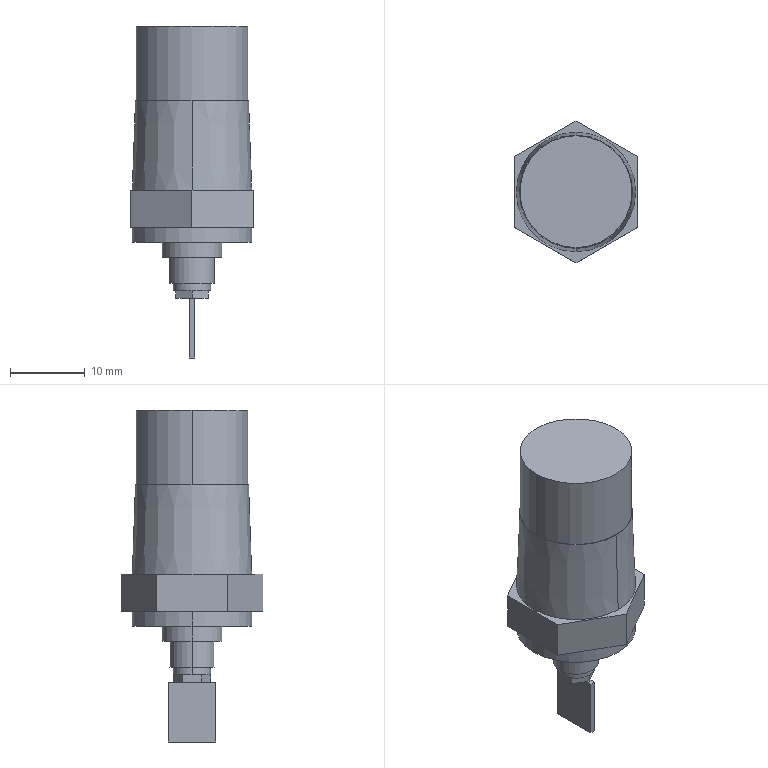Part | SolidWorks | features BaseBody 1 | 1 solid | 46 faces | box 16.454 x 19 x 44.5 mm | volume 5901 mm3 | plane 34 | cylinder 10 | cone 2 | commonest cylinder face diameters 5 x2 6 x2 8 x2 15 x2 16 x2
STEP:
#1=CARTESIAN_POINT('',(0.,7.581,0.));
#2=VERTEX_POINT('',#1);
#3=CARTESIAN_POINT('',(0.,-7.581,0.));
#4=VERTEX_POINT('',#3);
#5=CARTESIAN_POINT('',(0.,0.,0.));
#6=DIRECTION('',(0.,0.,-1.));
#7=DIRECTION('',(0.,1.,0.));
#8=AXIS2_PLACEMENT_3D('',#5,#6,#7);
#9=CIRCLE('',#8,7.581);
#10=EDGE_CURVE('',#2,#4,#9,.T.);
#11=ORIENTED_EDGE('',*,*,#10,.T.);
#12=CARTESIAN_POINT('',(0.,-8.,-12.));
#13=VERTEX_POINT('',#12);
#14=CARTESIAN_POINT('',(0.,-8.,-12.));
#15=DIRECTION('',(0.,-0.0349,-0.9994));
#16=VECTOR('',#15,1000.);
#17=LINE('',#14,#16);
#18=EDGE_CURVE('',#4,#13,#17,.T.);
#19=ORIENTED_EDGE('',*,*,#18,.T.);
#20=CARTESIAN_POINT('',(0.,8.,-12.));
#21=VERTEX_POINT('',#20);
#22=CARTESIAN_POINT('',(0.,0.,-12.));
#23=DIRECTION('',(0.,0.,1.));
#24=DIRECTION('',(0.,1.,0.));
#25=AXIS2_PLACEMENT_3D('',#22,#23,#24);
#26=CIRCLE('',#25,8.);
#27=EDGE_CURVE('',#13,#21,#26,.T.);
#28=ORIENTED_EDGE('',*,*,#27,.T.);
#29=CARTESIAN_POINT('',(0.,8.,-12.));
#30=DIRECTION('',(0.,0.0349,-0.9994));
#31=VECTOR('',#30,1000.);
#32=LINE('',#29,#31);
#33=EDGE_CURVE('',#2,#21,#32,.T.);
#34=ORIENTED_EDGE('',*,*,#33,.F.);
#35=EDGE_LOOP('',(#11,#19,#28,#34));
#36=FACE_OUTER_BOUND('',#35,.T.);
#37=CARTESIAN_POINT('',(0.,0.,-12.));
#38=DIRECTION('',(0.,0.,-1.));
#39=DIRECTION('',(0.,1.,0.));
#40=AXIS2_PLACEMENT_3D('',#37,#38,#39);
#41=CONICAL_SURFACE('',#40,8.,0.03491);
#42=ADVANCED_FACE('',(#36),#41,.T.);
#43=CARTESIAN_POINT('',(-7.5,0.,0.));
#44=VERTEX_POINT('',#43);
#45=CARTESIAN_POINT('',(7.5,0.,0.));
#46=VERTEX_POINT('',#45);
#47=CARTESIAN_POINT('',(0.,0.,0.));
#48=DIRECTION('',(0.,0.,-1.));
#49=DIRECTION('',(1.,0.,0.));
#50=AXIS2_PLACEMENT_3D('',#47,#48,#49);
#51=CIRCLE('',#50,7.5);
#52=EDGE_CURVE('',#44,#46,#51,.T.);
#53=ORIENTED_EDGE('',*,*,#52,.F.);
#54=CARTESIAN_POINT('',(-7.5,0.,10.));
#55=VERTEX_POINT('',#54);
#56=CARTESIAN_POINT('',(-7.5,0.,0.));
#57=DIRECTION('',(0.,0.,1.));
#58=VECTOR('',#57,1000.);
#59=LINE('',#56,#58);
#60=EDGE_CURVE('',#44,#55,#59,.T.);
#61=ORIENTED_EDGE('',*,*,#60,.T.);
#62=CARTESIAN_POINT('',(7.5,0.,10.));
#63=VERTEX_POINT('',#62);
#64=CARTESIAN_POINT('',(0.,0.,10.));
#65=DIRECTION('',(0.,0.,-1.));
#66=DIRECTION('',(1.,0.,0.));
#67=AXIS2_PLACEMENT_3D('',#64,#65,#66);
#68=CIRCLE('',#67,7.5);
#69=EDGE_CURVE('',#55,#63,#68,.T.);
#70=ORIENTED_EDGE('',*,*,#69,.T.);
#71=CARTESIAN_POINT('',(7.5,0.,0.));
#72=DIRECTION('',(0.,0.,1.));
#73=VECTOR('',#72,1000.);
#74=LINE('',#71,#73);
#75=EDGE_CURVE('',#46,#63,#74,.T.);
#76=ORIENTED_EDGE('',*,*,#75,.F.);
#77=EDGE_LOOP('',(#53,#61,#70,#76));
#78=FACE_OUTER_BOUND('',#77,.T.);
#79=CARTESIAN_POINT('',(0.,0.,0.));
#80=DIRECTION('',(0.,0.,1.));
#81=DIRECTION('',(1.,0.,0.));
#82=AXIS2_PLACEMENT_3D('',#79,#80,#81);
#83=CYLINDRICAL_SURFACE('',#82,7.5);
#84=ADVANCED_FACE('',(#78),#83,.T.);
#85=CARTESIAN_POINT('',(-8.,0.,-17.));
#86=VERTEX_POINT('',#85);
#87=CARTESIAN_POINT('',(8.,0.,-17.));
#88=VERTEX_POINT('',#87);
#89=CARTESIAN_POINT('',(0.,0.,-17.));
#90=DIRECTION('',(0.,0.,-1.));
#91=DIRECTION('',(-1.,0.,0.));
#92=AXIS2_PLACEMENT_3D('',#89,#90,#91);
#93=CIRCLE('',#92,8.);
#94=EDGE_CURVE('',#86,#88,#93,.T.);
#95=ORIENTED_EDGE('',*,*,#94,.T.);
#96=CARTESIAN_POINT('',(8.,0.,-19.));
#97=VERTEX_POINT('',#96);
#98=CARTESIAN_POINT('',(8.,0.,-17.));
#99=DIRECTION('',(0.,0.,-1.));
#100=VECTOR('',#99,1000.);
#101=LINE('',#98,#100);
#102=EDGE_CURVE('',#88,#97,#101,.T.);
#103=ORIENTED_EDGE('',*,*,#102,.T.);
#104=CARTESIAN_POINT('',(-8.,0.,-19.));
#105=VERTEX_POINT('',#104);
#106=CARTESIAN_POINT('',(0.,0.,-19.));
#107=DIRECTION('',(0.,0.,1.));
#108=DIRECTION('',(-1.,0.,0.));
#109=AXIS2_PLACEMENT_3D('',#106,#107,#108);
#110=CIRCLE('',#109,8.);
#111=EDGE_CURVE('',#97,#105,#110,.T.);
#112=ORIENTED_EDGE('',*,*,#111,.T.);
#113=CARTESIAN_POINT('',(-8.,0.,-17.));
#114=DIRECTION('',(0.,0.,-1.));
#115=VECTOR('',#114,1000.);
#116=LINE('',#113,#115);
#117=EDGE_CURVE('',#86,#105,#116,.T.);
#118=ORIENTED_EDGE('',*,*,#117,.F.);
#119=EDGE_LOOP('',(#95,#103,#112,#118));
#120=FACE_OUTER_BOUND('',#119,.T.);
#121=CARTESIAN_POINT('',(0.,0.,-17.));
#122=DIRECTION('',(0.,0.,-1.));
#123=DIRECTION('',(-1.,0.,0.));
#124=AXIS2_PLACEMENT_3D('',#121,#122,#123);
#125=CYLINDRICAL_SURFACE('',#124,8.);
#126=ADVANCED_FACE('',(#120),#125,.T.);
#127=CARTESIAN_POINT('',(-4.,0.,-19.));
#128=VERTEX_POINT('',#127);
#129=CARTESIAN_POINT('',(4.,0.,-19.));
#130=VERTEX_POINT('',#129);
#131=CARTESIAN_POINT('',(0.,0.,-19.));
#132=DIRECTION('',(0.,0.,-1.));
#133=DIRECTION('',(-1.,0.,0.));
#134=AXIS2_PLACEMENT_3D('',#131,#132,#133);
#135=CIRCLE('',#134,4.);
#136=EDGE_CURVE('',#128,#130,#135,.T.);
#137=ORIENTED_EDGE('',*,*,#136,.T.);
#138=CARTESIAN_POINT('',(4.,0.,-21.));
#139=VERTEX_POINT('',#138);
#140=CARTESIAN_POINT('',(4.,0.,-19.));
#141=DIRECTION('',(0.,0.,-1.));
#142=VECTOR('',#141,1000.);
#143=LINE('',#140,#142);
#144=EDGE_CURVE('',#130,#139,#143,.T.);
#145=ORIENTED_EDGE('',*,*,#144,.T.);
#146=CARTESIAN_POINT('',(-4.,0.,-21.));
#147=VERTEX_POINT('',#146);
#148=CARTESIAN_POINT('',(0.,0.,-21.));
#149=DIRECTION('',(0.,0.,1.));
#150=DIRECTION('',(-1.,0.,0.));
#151=AXIS2_PLACEMENT_3D('',#148,#149,#150);
#152=CIRCLE('',#151,4.);
#153=EDGE_CURVE('',#139,#147,#152,.T.);
#154=ORIENTED_EDGE('',*,*,#153,.T.);
#155=CARTESIAN_POINT('',(-4.,0.,-19.));
#156=DIRECTION('',(0.,0.,-1.));
#157=VECTOR('',#156,1000.);
#158=LINE('',#155,#157);
#159=EDGE_CURVE('',#128,#147,#158,.T.);
#160=ORIENTED_EDGE('',*,*,#159,.F.);
#161=EDGE_LOOP('',(#137,#145,#154,#160));
#162=FACE_OUTER_BOUND('',#161,.T.);
#163=CARTESIAN_POINT('',(0.,0.,-19.));
#164=DIRECTION('',(0.,0.,-1.));
#165=DIRECTION('',(-1.,0.,0.));
#166=AXIS2_PLACEMENT_3D('',#163,#164,#165);
#167=CYLINDRICAL_SURFACE('',#166,4.);
#168=ADVANCED_FACE('',(#162),#167,.T.);
#169=CARTESIAN_POINT('',(-3.,0.,-21.));
#170=VERTEX_POINT('',#169);
#171=CARTESIAN_POINT('',(3.,0.,-21.));
#172=VERTEX_POINT('',#171);
#173=CARTESIAN_POINT('',(0.,0.,-21.));
#174=DIRECTION('',(0.,0.,-1.));
#175=DIRECTION('',(-1.,0.,0.));
#176=AXIS2_PLACEMENT_3D('',#173,#174,#175);
#177=CIRCLE('',#176,3.);
#178=EDGE_CURVE('',#170,#172,#177,.T.);
#179=ORIENTED_EDGE('',*,*,#178,.T.);
#180=CARTESIAN_POINT('',(3.,0.,-24.5));
#181=VERTEX_POINT('',#180);
#182=CARTESIAN_POINT('',(3.,0.,-21.));
#183=DIRECTION('',(0.,0.,-1.));
#184=VECTOR('',#183,1000.);
#185=LINE('',#182,#184);
#186=EDGE_CURVE('',#172,#181,#185,.T.);
#187=ORIENTED_EDGE('',*,*,#186,.T.);
#188=CARTESIAN_POINT('',(-3.,0.,-24.5));
#189=VERTEX_POINT('',#188);
#190=CARTESIAN_POINT('',(0.,0.,-24.5));
#191=DIRECTION('',(0.,0.,1.));
#192=DIRECTION('',(-1.,0.,0.));
#193=AXIS2_PLACEMENT_3D('',#190,#191,#192);
#194=CIRCLE('',#193,3.);
#195=EDGE_CURVE('',#181,#189,#194,.T.);
#196=ORIENTED_EDGE('',*,*,#195,.T.);
#197=CARTESIAN_POINT('',(-3.,0.,-21.));
#198=DIRECTION('',(0.,0.,-1.));
#199=VECTOR('',#198,1000.);
#200=LINE('',#197,#199);
#201=EDGE_CURVE('',#170,#189,#200,.T.);
#202=ORIENTED_EDGE('',*,*,#201,.F.);
#203=EDGE_LOOP('',(#179,#187,#196,#202));
#204=FACE_OUTER_BOUND('',#203,.T.);
#205=CARTESIAN_POINT('',(0.,0.,-21.));
#206=DIRECTION('',(0.,0.,-1.));
#207=DIRECTION('',(-1.,0.,0.));
#208=AXIS2_PLACEMENT_3D('',#205,#206,#207);
#209=CYLINDRICAL_SURFACE('',#208,3.);
#210=ADVANCED_FACE('',(#204),#209,.T.);
#211=CARTESIAN_POINT('',(-2.5,0.,-24.5));
#212=VERTEX_POINT('',#211);
#213=CARTESIAN_POINT('',(2.5,0.,-24.5));
#214=VERTEX_POINT('',#213);
#215=CARTESIAN_POINT('',(0.,0.,-24.5));
#216=DIRECTION('',(0.,0.,-1.));
#217=DIRECTION('',(-1.,0.,0.));
#218=AXIS2_PLACEMENT_3D('',#215,#216,#217);
#219=CIRCLE('',#218,2.5);
#220=EDGE_CURVE('',#212,#214,#219,.T.);
#221=ORIENTED_EDGE('',*,*,#220,.T.);
#222=CARTESIAN_POINT('',(2.5,0.,-25.5));
#223=VERTEX_POINT('',#222);
#224=CARTESIAN_POINT('',(2.5,0.,-24.5));
#225=DIRECTION('',(0.,0.,-1.));
#226=VECTOR('',#225,1000.);
#227=LINE('',#224,#226);
#228=EDGE_CURVE('',#214,#223,#227,.T.);
#229=ORIENTED_EDGE('',*,*,#228,.T.);
#230=CARTESIAN_POINT('',(2.165,1.25,-25.5));
#231=VERTEX_POINT('',#230);
#232=CARTESIAN_POINT('',(0.,0.,-25.5));
#233=DIRECTION('',(0.,0.,1.));
#234=DIRECTION('',(-1.,0.,0.));
#235=AXIS2_PLACEMENT_3D('',#232,#233,#234);
#236=CIRCLE('',#235,2.5);
#237=EDGE_CURVE('',#223,#231,#236,.T.);
#238=ORIENTED_EDGE('',*,*,#237,.T.);
#239=CARTESIAN_POINT('',(0.,2.5,-25.5));
#240=VERTEX_POINT('',#239);
#241=CARTESIAN_POINT('',(0.,0.,-25.5));
#242=DIRECTION('',(0.,0.,1.));
#243=DIRECTION('',(-1.,0.,0.));
#244=AXIS2_PLACEMENT_3D('',#241,#242,#243);
#245=CIRCLE('',#244,2.5);
#246=EDGE_CURVE('',#231,#240,#245,.T.);
#247=ORIENTED_EDGE('',*,*,#246,.T.);
#248=CARTESIAN_POINT('',(-2.165,1.25,-25.5));
#249=VERTEX_POINT('',#248);
#250=CARTESIAN_POINT('',(0.,0.,-25.5));
#251=DIRECTION('',(0.,0.,1.));
#252=DIRECTION('',(-1.,0.,0.));
#253=AXIS2_PLACEMENT_3D('',#250,#251,#252);
#254=CIRCLE('',#253,2.5);
#255=EDGE_CURVE('',#240,#249,#254,.T.);
#256=ORIENTED_EDGE('',*,*,#255,.T.);
#257=CARTESIAN_POINT('',(-2.5,0.,-25.5));
#258=VERTEX_POINT('',#257);
#259=CARTESIAN_POINT('',(0.,0.,-25.5));
#260=DIRECTION('',(0.,0.,1.));
#261=DIRECTION('',(-1.,0.,0.));
#262=AXIS2_PLACEMENT_3D('',#259,#260,#261);
#263=CIRCLE('',#262,2.5);
#264=EDGE_CURVE('',#249,#258,#263,.T.);
#265=ORIENTED_EDGE('',*,*,#264,.T.);
#266=CARTESIAN_POINT('',(-2.5,0.,-24.5));
#267=DIRECTION('',(0.,0.,-1.));
#268=VECTOR('',#267,1000.);
#269=LINE('',#266,#268);
#270=EDGE_CURVE('',#212,#258,#269,.T.);
#271=ORIENTED_EDGE('',*,*,#270,.F.);
#272=EDGE_LOOP('',(#221,#229,#238,#247,#256,#265,#271));
#273=FACE_OUTER_BOUND('',#272,.T.);
#274=CARTESIAN_POINT('',(0.,0.,-24.5));
#275=DIRECTION('',(0.,0.,-1.));
#276=DIRECTION('',(-1.,0.,0.));
#277=AXIS2_PLACEMENT_3D('',#274,#275,#276);
#278=CYLINDRICAL_SURFACE('',#277,2.5);
#279=ADVANCED_FACE('',(#273),#278,.T.);
#280=ORIENTED_EDGE('',*,*,#18,.F.);
#281=CARTESIAN_POINT('',(0.,0.,0.));
#282=DIRECTION('',(0.,0.,-1.));
#283=DIRECTION('',(0.,1.,0.));
#284=AXIS2_PLACEMENT_3D('',#281,#282,#283);
#285=CIRCLE('',#284,7.581);
#286=EDGE_CURVE('',#4,#2,#285,.T.);
#287=ORIENTED_EDGE('',*,*,#286,.T.);
#288=ORIENTED_EDGE('',*,*,#33,.T.);
#289=CARTESIAN_POINT('',(0.,0.,-12.));
#290=DIRECTION('',(0.,0.,1.));
#291=DIRECTION('',(0.,1.,0.));
#292=AXIS2_PLACEMENT_3D('',#289,#290,#291);
#293=CIRCLE('',#292,8.);
#294=EDGE_CURVE('',#21,#13,#293,.T.);
#295=ORIENTED_EDGE('',*,*,#294,.T.);
#296=EDGE_LOOP('',(#280,#287,#288,#295));
#297=FACE_OUTER_BOUND('',#296,.T.);
#298=CARTESIAN_POINT('',(0.,0.,-12.));
#299=DIRECTION('',(0.,0.,-1.));
#300=DIRECTION('',(0.,1.,0.));
#301=AXIS2_PLACEMENT_3D('',#298,#299,#300);
#302=CONICAL_SURFACE('',#301,8.,0.03491);
#303=ADVANCED_FACE('',(#297),#302,.T.);
#304=CARTESIAN_POINT('',(0.,0.,0.));
#305=DIRECTION('',(0.,0.,-1.));
#306=DIRECTION('',(1.,0.,0.));
#307=AXIS2_PLACEMENT_3D('',#304,#305,#306);
#308=CIRCLE('',#307,7.5);
#309=EDGE_CURVE('',#46,#44,#308,.T.);
#310=ORIENTED_EDGE('',*,*,#309,.T.);
#311=ORIENTED_EDGE('',*,*,#52,.T.);
#312=EDGE_LOOP('',(#310,#311));
#313=FACE_BOUND('',#312,.T.);
#314=ORIENTED_EDGE('',*,*,#10,.F.);
#315=ORIENTED_EDGE('',*,*,#286,.F.);
#316=EDGE_LOOP('',(#314,#315));
#317=FACE_OUTER_BOUND('',#316,.T.);
#318=CARTESIAN_POINT('',(0.,0.,0.));
#319=DIRECTION('',(0.,0.,1.));
#320=DIRECTION('',(1.,0.,0.));
#321=AXIS2_PLACEMENT_3D('',#318,#319,#320);
#322=PLANE('',#321);
#323=ADVANCED_FACE('',(#313,#317),#322,.T.);
#324=ORIENTED_EDGE('',*,*,#294,.F.);
#325=ORIENTED_EDGE('',*,*,#27,.F.);
#326=EDGE_LOOP('',(#324,#325));
#327=FACE_BOUND('',#326,.T.);
#328=CARTESIAN_POINT('',(-8.227,-4.75,-12.));
#329=VERTEX_POINT('',#328);
#330=CARTESIAN_POINT('',(-0.000000001,-9.5,-12.));
#331=VERTEX_POINT('',#330);
#332=CARTESIAN_POINT('',(-8.227,-4.75,-12.));
#333=DIRECTION('',(0.866,-0.5,0.));
#334=VECTOR('',#333,1000.);
#335=LINE('',#332,#334);
#336=EDGE_CURVE('',#329,#331,#335,.T.);
#337=ORIENTED_EDGE('',*,*,#336,.T.);
#338=CARTESIAN_POINT('',(8.227,-4.75,-12.));
#339=VERTEX_POINT('',#338);
#340=CARTESIAN_POINT('',(-0.000000001,-9.5,-12.));
#341=DIRECTION('',(0.866,0.5,0.));
#342=VECTOR('',#341,1000.);
#343=LINE('',#340,#342);
#344=EDGE_CURVE('',#331,#339,#343,.T.);
#345=ORIENTED_EDGE('',*,*,#344,.T.);
#346=CARTESIAN_POINT('',(8.227,4.75,-12.));
#347=VERTEX_POINT('',#346);
#348=CARTESIAN_POINT('',(8.227,0.,-12.));
#349=DIRECTION('',(0.,1.,0.));
#350=VECTOR('',#349,1000.);
#351=LINE('',#348,#350);
#352=EDGE_CURVE('',#339,#347,#351,.T.);
#353=ORIENTED_EDGE('',*,*,#352,.T.);
#354=CARTESIAN_POINT('',(0.000000001,9.5,-12.));
#355=VERTEX_POINT('',#354);
#356=CARTESIAN_POINT('',(8.227,4.75,-12.));
#357=DIRECTION('',(-0.866,0.5,0.));
#358=VECTOR('',#357,1000.);
#359=LINE('',#356,#358);
#360=EDGE_CURVE('',#347,#355,#359,.T.);
#361=ORIENTED_EDGE('',*,*,#360,.T.);
#362=CARTESIAN_POINT('',(-8.227,4.75,-12.));
#363=VERTEX_POINT('',#362);
#364=CARTESIAN_POINT('',(0.000000001,9.5,-12.));
#365=DIRECTION('',(-0.866,-0.5,0.));
#366=VECTOR('',#365,1000.);
#367=LINE('',#364,#366);
#368=EDGE_CURVE('',#355,#363,#367,.T.);
#369=ORIENTED_EDGE('',*,*,#368,.T.);
#370=CARTESIAN_POINT('',(-8.227,0.,-12.));
#371=DIRECTION('',(0.,-1.,0.));
#372=VECTOR('',#371,1000.);
#373=LINE('',#370,#372);
#374=EDGE_CURVE('',#363,#329,#373,.T.);
#375=ORIENTED_EDGE('',*,*,#374,.T.);
#376=EDGE_LOOP('',(#337,#345,#353,#361,#369,#375));
#377=FACE_OUTER_BOUND('',#376,.T.);
#378=CARTESIAN_POINT('',(0.,0.,-12.));
#379=DIRECTION('',(0.,0.,1.));
#380=DIRECTION('',(1.,0.,0.));
#381=AXIS2_PLACEMENT_3D('',#378,#379,#380);
#382=PLANE('',#381);
#383=ADVANCED_FACE('',(#327,#377),#382,.T.);
#384=ORIENTED_EDGE('',*,*,#60,.F.);
#385=ORIENTED_EDGE('',*,*,#309,.F.);
#386=ORIENTED_EDGE('',*,*,#75,.T.);
#387=CARTESIAN_POINT('',(0.,0.,10.));
#388=DIRECTION('',(0.,0.,-1.));
#389=DIRECTION('',(1.,0.,0.));
#390=AXIS2_PLACEMENT_3D('',#387,#388,#389);
#391=CIRCLE('',#390,7.5);
#392=EDGE_CURVE('',#63,#55,#391,.T.);
#393=ORIENTED_EDGE('',*,*,#392,.T.);
#394=EDGE_LOOP('',(#384,#385,#386,#393));
#395=FACE_OUTER_BOUND('',#394,.T.);
#396=CARTESIAN_POINT('',(0.,0.,0.));
#397=DIRECTION('',(0.,0.,1.));
#398=DIRECTION('',(1.,0.,0.));
#399=AXIS2_PLACEMENT_3D('',#396,#397,#398);
#400=CYLINDRICAL_SURFACE('',#399,7.5);
#401=ADVANCED_FACE('',(#395),#400,.T.);
#402=CARTESIAN_POINT('',(8.227,-4.75,-17.));
#403=VERTEX_POINT('',#402);
#404=CARTESIAN_POINT('',(8.227,-4.75,-14.5));
#405=DIRECTION('',(0.,0.,-1.));
#406=VECTOR('',#405,1000.);
#407=LINE('',#404,#406);
#408=EDGE_CURVE('',#339,#403,#407,.T.);
#409=ORIENTED_EDGE('',*,*,#408,.F.);
#410=ORIENTED_EDGE('',*,*,#344,.F.);
#411=CARTESIAN_POINT('',(-0.000000001,-9.5,-17.));
#412=VERTEX_POINT('',#411);
#413=CARTESIAN_POINT('',(0.000000001,-9.5,-14.5));
#414=DIRECTION('',(0.,0.,1.));
#415=VECTOR('',#414,1000.);
#416=LINE('',#413,#415);
#417=EDGE_CURVE('',#412,#331,#416,.T.);
#418=ORIENTED_EDGE('',*,*,#417,.F.);
#419=CARTESIAN_POINT('',(4.114,-7.125,-17.));
#420=DIRECTION('',(-0.866,-0.5,0.));
#421=VECTOR('',#420,1000.);
#422=LINE('',#419,#421);
#423=EDGE_CURVE('',#403,#412,#422,.T.);
#424=ORIENTED_EDGE('',*,*,#423,.F.);
#425=EDGE_LOOP('',(#409,#410,#418,#424));
#426=FACE_OUTER_BOUND('',#425,.T.);
#427=CARTESIAN_POINT('',(4.114,-7.125,-14.5));
#428=DIRECTION('',(-0.5,0.866,0.));
#429=DIRECTION('',(-0.866,-0.5,0.));
#430=AXIS2_PLACEMENT_3D('',#427,#428,#429);
#431=PLANE('',#430);
#432=ADVANCED_FACE('',(#426),#431,.F.);
#433=ORIENTED_EDGE('',*,*,#417,.T.);
#434=ORIENTED_EDGE('',*,*,#336,.F.);
#435=CARTESIAN_POINT('',(-8.227,-4.75,-17.));
#436=VERTEX_POINT('',#435);
#437=CARTESIAN_POINT('',(-8.227,-4.75,-14.5));
#438=DIRECTION('',(0.,0.,1.));
#439=VECTOR('',#438,1000.);
#440=LINE('',#437,#439);
#441=EDGE_CURVE('',#436,#329,#440,.T.);
#442=ORIENTED_EDGE('',*,*,#441,.F.);
#443=CARTESIAN_POINT('',(-4.114,-7.125,-17.));
#444=DIRECTION('',(-0.866,0.5,0.));
#445=VECTOR('',#444,1000.);
#446=LINE('',#443,#445);
#447=EDGE_CURVE('',#412,#436,#446,.T.);
#448=ORIENTED_EDGE('',*,*,#447,.F.);
#449=EDGE_LOOP('',(#433,#434,#442,#448));
#450=FACE_OUTER_BOUND('',#449,.T.);
#451=CARTESIAN_POINT('',(-4.114,-7.125,-14.5));
#452=DIRECTION('',(0.5,0.866,0.));
#453=DIRECTION('',(-0.866,0.5,0.));
#454=AXIS2_PLACEMENT_3D('',#451,#452,#453);
#455=PLANE('',#454);
#456=ADVANCED_FACE('',(#450),#455,.F.);
#457=ORIENTED_EDGE('',*,*,#441,.T.);
#458=ORIENTED_EDGE('',*,*,#374,.F.);
#459=CARTESIAN_POINT('',(-8.227,4.75,-17.));
#460=VERTEX_POINT('',#459);
#461=CARTESIAN_POINT('',(-8.227,4.75,-14.5));
#462=DIRECTION('',(0.,0.,1.));
#463=VECTOR('',#462,1000.);
#464=LINE('',#461,#463);
#465=EDGE_CURVE('',#460,#363,#464,.T.);
#466=ORIENTED_EDGE('',*,*,#465,.F.);
#467=CARTESIAN_POINT('',(-8.227,0.,-17.));
#468=DIRECTION('',(0.,1.,0.));
#469=VECTOR('',#468,1000.);
#470=LINE('',#467,#469);
#471=EDGE_CURVE('',#436,#460,#470,.T.);
#472=ORIENTED_EDGE('',*,*,#471,.F.);
#473=EDGE_LOOP('',(#457,#458,#466,#472));
#474=FACE_OUTER_BOUND('',#473,.T.);
#475=CARTESIAN_POINT('',(-8.227,0.,-14.5));
#476=DIRECTION('',(1.,0.,0.));
#477=DIRECTION('',(0.,0.,-1.));
#478=AXIS2_PLACEMENT_3D('',#475,#476,#477);
#479=PLANE('',#478);
#480=ADVANCED_FACE('',(#474),#479,.F.);
#481=ORIENTED_EDGE('',*,*,#368,.F.);
#482=CARTESIAN_POINT('',(0.000000001,9.5,-17.));
#483=VERTEX_POINT('',#482);
#484=CARTESIAN_POINT('',(0.,9.5,-14.5));
#485=DIRECTION('',(0.,0.,-1.));
#486=VECTOR('',#485,1000.);
#487=LINE('',#484,#486);
#488=EDGE_CURVE('',#355,#483,#487,.T.);
#489=ORIENTED_EDGE('',*,*,#488,.T.);
#490=CARTESIAN_POINT('',(-4.114,7.125,-17.));
#491=DIRECTION('',(-0.866,-0.5,0.));
#492=VECTOR('',#491,1000.);
#493=LINE('',#490,#492);
#494=EDGE_CURVE('',#483,#460,#493,.T.);
#495=ORIENTED_EDGE('',*,*,#494,.T.);
#496=ORIENTED_EDGE('',*,*,#465,.T.);
#497=EDGE_LOOP('',(#481,#489,#495,#496));
#498=FACE_OUTER_BOUND('',#497,.T.);
#499=CARTESIAN_POINT('',(-4.114,7.125,-14.5));
#500=DIRECTION('',(-0.5,0.866,0.));
#501=DIRECTION('',(-0.866,-0.5,0.));
#502=AXIS2_PLACEMENT_3D('',#499,#500,#501);
#503=PLANE('',#502);
#504=ADVANCED_FACE('',(#498),#503,.T.);
#505=ORIENTED_EDGE('',*,*,#360,.F.);
#506=CARTESIAN_POINT('',(8.227,4.75,-17.));
#507=VERTEX_POINT('',#506);
#508=CARTESIAN_POINT('',(8.227,4.75,-14.5));
#509=DIRECTION('',(0.,0.,-1.));
#510=VECTOR('',#509,1000.);
#511=LINE('',#508,#510);
#512=EDGE_CURVE('',#347,#507,#511,.T.);
#513=ORIENTED_EDGE('',*,*,#512,.T.);
#514=CARTESIAN_POINT('',(4.114,7.125,-17.));
#515=DIRECTION('',(-0.866,0.5,0.));
#516=VECTOR('',#515,1000.);
#517=LINE('',#514,#516);
#518=EDGE_CURVE('',#507,#483,#517,.T.);
#519=ORIENTED_EDGE('',*,*,#518,.T.);
#520=ORIENTED_EDGE('',*,*,#488,.F.);
#521=EDGE_LOOP('',(#505,#513,#519,#520));
#522=FACE_OUTER_BOUND('',#521,.T.);
#523=CARTESIAN_POINT('',(4.114,7.125,-14.5));
#524=DIRECTION('',(0.5,0.866,0.));
#525=DIRECTION('',(-0.866,0.5,0.));
#526=AXIS2_PLACEMENT_3D('',#523,#524,#525);
#527=PLANE('',#526);
#528=ADVANCED_FACE('',(#522),#527,.T.);
#529=ORIENTED_EDGE('',*,*,#352,.F.);
#530=ORIENTED_EDGE('',*,*,#408,.T.);
#531=CARTESIAN_POINT('',(8.227,0.,-17.));
#532=DIRECTION('',(0.,1.,0.));
#533=VECTOR('',#532,1000.);
#534=LINE('',#531,#533);
#535=EDGE_CURVE('',#403,#507,#534,.T.);
#536=ORIENTED_EDGE('',*,*,#535,.T.);
#537=ORIENTED_EDGE('',*,*,#512,.F.);
#538=EDGE_LOOP('',(#529,#530,#536,#537));
#539=FACE_OUTER_BOUND('',#538,.T.);
#540=CARTESIAN_POINT('',(8.227,0.,-14.5));
#541=DIRECTION('',(1.,0.,0.));
#542=DIRECTION('',(0.,0.,-1.));
#543=AXIS2_PLACEMENT_3D('',#540,#541,#542);
#544=PLANE('',#543);
#545=ADVANCED_FACE('',(#539),#544,.T.);
#546=ORIENTED_EDGE('',*,*,#392,.F.);
#547=ORIENTED_EDGE('',*,*,#69,.F.);
#548=EDGE_LOOP('',(#546,#547));
#549=FACE_OUTER_BOUND('',#548,.T.);
#550=CARTESIAN_POINT('',(0.,0.,10.));
#551=DIRECTION('',(0.,0.,1.));
#552=DIRECTION('',(1.,0.,0.));
#553=AXIS2_PLACEMENT_3D('',#550,#551,#552);
#554=PLANE('',#553);
#555=ADVANCED_FACE('',(#549),#554,.T.);
#556=ORIENTED_EDGE('',*,*,#94,.F.);
#557=CARTESIAN_POINT('',(0.,0.,-17.));
#558=DIRECTION('',(0.,0.,-1.));
#559=DIRECTION('',(-1.,0.,0.));
#560=AXIS2_PLACEMENT_3D('',#557,#558,#559);
#561=CIRCLE('',#560,8.);
#562=EDGE_CURVE('',#88,#86,#561,.T.);
#563=ORIENTED_EDGE('',*,*,#562,.F.);
#564=EDGE_LOOP('',(#556,#563));
#565=FACE_BOUND('',#564,.T.);
#566=ORIENTED_EDGE('',*,*,#447,.T.);
#567=ORIENTED_EDGE('',*,*,#471,.T.);
#568=ORIENTED_EDGE('',*,*,#494,.F.);
#569=ORIENTED_EDGE('',*,*,#518,.F.);
#570=ORIENTED_EDGE('',*,*,#535,.F.);
#571=ORIENTED_EDGE('',*,*,#423,.T.);
#572=EDGE_LOOP('',(#566,#567,#568,#569,#570,#571));
#573=FACE_OUTER_BOUND('',#572,.T.);
#574=CARTESIAN_POINT('',(0.,0.,-17.));
#575=DIRECTION('',(0.,0.,1.));
#576=DIRECTION('',(1.,0.,0.));
#577=AXIS2_PLACEMENT_3D('',#574,#575,#576);
#578=PLANE('',#577);
#579=ADVANCED_FACE('',(#565,#573),#578,.F.);
#580=ORIENTED_EDGE('',*,*,#102,.F.);
#581=ORIENTED_EDGE('',*,*,#562,.T.);
#582=ORIENTED_EDGE('',*,*,#117,.T.);
#583=CARTESIAN_POINT('',(0.,0.,-19.));
#584=DIRECTION('',(0.,0.,1.));
#585=DIRECTION('',(-1.,0.,0.));
#586=AXIS2_PLACEMENT_3D('',#583,#584,#585);
#587=CIRCLE('',#586,8.);
#588=EDGE_CURVE('',#105,#97,#587,.T.);
#589=ORIENTED_EDGE('',*,*,#588,.T.);
#590=EDGE_LOOP('',(#580,#581,#582,#589));
#591=FACE_OUTER_BOUND('',#590,.T.);
#592=CARTESIAN_POINT('',(0.,0.,-17.));
#593=DIRECTION('',(0.,0.,-1.));
#594=DIRECTION('',(-1.,0.,0.));
#595=AXIS2_PLACEMENT_3D('',#592,#593,#594);
#596=CYLINDRICAL_SURFACE('',#595,8.);
#597=ADVANCED_FACE('',(#591),#596,.T.);
#598=ORIENTED_EDGE('',*,*,#136,.F.);
#599=CARTESIAN_POINT('',(0.,0.,-19.));
#600=DIRECTION('',(0.,0.,-1.));
#601=DIRECTION('',(-1.,0.,0.));
#602=AXIS2_PLACEMENT_3D('',#599,#600,#601);
#603=CIRCLE('',#602,4.);
#604=EDGE_CURVE('',#130,#128,#603,.T.);
#605=ORIENTED_EDGE('',*,*,#604,.F.);
#606=EDGE_LOOP('',(#598,#605));
#607=FACE_BOUND('',#606,.T.);
#608=ORIENTED_EDGE('',*,*,#588,.F.);
#609=ORIENTED_EDGE('',*,*,#111,.F.);
#610=EDGE_LOOP('',(#608,#609));
#611=FACE_OUTER_BOUND('',#610,.T.);
#612=CARTESIAN_POINT('',(0.,0.,-19.));
#613=DIRECTION('',(0.,0.,1.));
#614=DIRECTION('',(1.,0.,0.));
#615=AXIS2_PLACEMENT_3D('',#612,#613,#614);
#616=PLANE('',#615);
#617=ADVANCED_FACE('',(#607,#611),#616,.F.);
#618=ORIENTED_EDGE('',*,*,#144,.F.);
#619=ORIENTED_EDGE('',*,*,#604,.T.);
#620=ORIENTED_EDGE('',*,*,#159,.T.);
#621=CARTESIAN_POINT('',(0.,0.,-21.));
#622=DIRECTION('',(0.,0.,1.));
#623=DIRECTION('',(-1.,0.,0.));
#624=AXIS2_PLACEMENT_3D('',#621,#622,#623);
#625=CIRCLE('',#624,4.);
#626=EDGE_CURVE('',#147,#139,#625,.T.);
#627=ORIENTED_EDGE('',*,*,#626,.T.);
#628=EDGE_LOOP('',(#618,#619,#620,#627));
#629=FACE_OUTER_BOUND('',#628,.T.);
#630=CARTESIAN_POINT('',(0.,0.,-19.));
#631=DIRECTION('',(0.,0.,-1.));
#632=DIRECTION('',(-1.,0.,0.));
#633=AXIS2_PLACEMENT_3D('',#630,#631,#632);
#634=CYLINDRICAL_SURFACE('',#633,4.);
#635=ADVANCED_FACE('',(#629),#634,.T.);
#636=ORIENTED_EDGE('',*,*,#178,.F.);
#637=CARTESIAN_POINT('',(0.,0.,-21.));
#638=DIRECTION('',(0.,0.,-1.));
#639=DIRECTION('',(-1.,0.,0.));
#640=AXIS2_PLACEMENT_3D('',#637,#638,#639);
#641=CIRCLE('',#640,3.);
#642=EDGE_CURVE('',#172,#170,#641,.T.);
#643=ORIENTED_EDGE('',*,*,#642,.F.);
#644=EDGE_LOOP('',(#636,#643));
#645=FACE_BOUND('',#644,.T.);
#646=ORIENTED_EDGE('',*,*,#626,.F.);
#647=ORIENTED_EDGE('',*,*,#153,.F.);
#648=EDGE_LOOP('',(#646,#647));
#649=FACE_OUTER_BOUND('',#648,.T.);
#650=CARTESIAN_POINT('',(0.,0.,-21.));
#651=DIRECTION('',(0.,0.,1.));
#652=DIRECTION('',(1.,0.,0.));
#653=AXIS2_PLACEMENT_3D('',#650,#651,#652);
#654=PLANE('',#653);
#655=ADVANCED_FACE('',(#645,#649),#654,.F.);
#656=ORIENTED_EDGE('',*,*,#186,.F.);
#657=ORIENTED_EDGE('',*,*,#642,.T.);
#658=ORIENTED_EDGE('',*,*,#201,.T.);
#659=CARTESIAN_POINT('',(0.,0.,-24.5));
#660=DIRECTION('',(0.,0.,1.));
#661=DIRECTION('',(-1.,0.,0.));
#662=AXIS2_PLACEMENT_3D('',#659,#660,#661);
#663=CIRCLE('',#662,3.);
#664=EDGE_CURVE('',#189,#181,#663,.T.);
#665=ORIENTED_EDGE('',*,*,#664,.T.);
#666=EDGE_LOOP('',(#656,#657,#658,#665));
#667=FACE_OUTER_BOUND('',#666,.T.);
#668=CARTESIAN_POINT('',(0.,0.,-21.));
#669=DIRECTION('',(0.,0.,-1.));
#670=DIRECTION('',(-1.,0.,0.));
#671=AXIS2_PLACEMENT_3D('',#668,#669,#670);
#672=CYLINDRICAL_SURFACE('',#671,3.);
#673=ADVANCED_FACE('',(#667),#672,.T.);
#674=ORIENTED_EDGE('',*,*,#220,.F.);
#675=CARTESIAN_POINT('',(0.,0.,-24.5));
#676=DIRECTION('',(0.,0.,-1.));
#677=DIRECTION('',(-1.,0.,0.));
#678=AXIS2_PLACEMENT_3D('',#675,#676,#677);
#679=CIRCLE('',#678,2.5);
#680=EDGE_CURVE('',#214,#212,#679,.T.);
#681=ORIENTED_EDGE('',*,*,#680,.F.);
#682=EDGE_LOOP('',(#674,#681));
#683=FACE_BOUND('',#682,.T.);
#684=ORIENTED_EDGE('',*,*,#664,.F.);
#685=ORIENTED_EDGE('',*,*,#195,.F.);
#686=EDGE_LOOP('',(#684,#685));
#687=FACE_OUTER_BOUND('',#686,.T.);
#688=CARTESIAN_POINT('',(0.,0.,-24.5));
#689=DIRECTION('',(0.,0.,1.));
#690=DIRECTION('',(1.,0.,0.));
#691=AXIS2_PLACEMENT_3D('',#688,#689,#690);
#692=PLANE('',#691);
#693=ADVANCED_FACE('',(#683,#687),#692,.F.);
#694=ORIENTED_EDGE('',*,*,#228,.F.);
#695=ORIENTED_EDGE('',*,*,#680,.T.);
#696=ORIENTED_EDGE('',*,*,#270,.T.);
#697=CARTESIAN_POINT('',(-2.165,-1.25,-25.5));
#698=VERTEX_POINT('',#697);
#699=CARTESIAN_POINT('',(0.,0.,-25.5));
#700=DIRECTION('',(0.,0.,1.));
#701=DIRECTION('',(-1.,0.,0.));
#702=AXIS2_PLACEMENT_3D('',#699,#700,#701);
#703=CIRCLE('',#702,2.5);
#704=EDGE_CURVE('',#258,#698,#703,.T.);
#705=ORIENTED_EDGE('',*,*,#704,.T.);
#706=CARTESIAN_POINT('',(0.,-2.5,-25.5));
#707=VERTEX_POINT('',#706);
#708=CARTESIAN_POINT('',(0.,0.,-25.5));
#709=DIRECTION('',(0.,0.,1.));
#710=DIRECTION('',(-1.,0.,0.));
#711=AXIS2_PLACEMENT_3D('',#708,#709,#710);
#712=CIRCLE('',#711,2.5);
#713=EDGE_CURVE('',#698,#707,#712,.T.);
#714=ORIENTED_EDGE('',*,*,#713,.T.);
#715=CARTESIAN_POINT('',(2.165,-1.25,-25.5));
#716=VERTEX_POINT('',#715);
#717=CARTESIAN_POINT('',(0.,0.,-25.5));
#718=DIRECTION('',(0.,0.,1.));
#719=DIRECTION('',(-1.,0.,0.));
#720=AXIS2_PLACEMENT_3D('',#717,#718,#719);
#721=CIRCLE('',#720,2.5);
#722=EDGE_CURVE('',#707,#716,#721,.T.);
#723=ORIENTED_EDGE('',*,*,#722,.T.);
#724=CARTESIAN_POINT('',(0.,0.,-25.5));
#725=DIRECTION('',(0.,0.,1.));
#726=DIRECTION('',(-1.,0.,0.));
#727=AXIS2_PLACEMENT_3D('',#724,#725,#726);
#728=CIRCLE('',#727,2.5);
#729=EDGE_CURVE('',#716,#223,#728,.T.);
#730=ORIENTED_EDGE('',*,*,#729,.T.);
#731=EDGE_LOOP('',(#694,#695,#696,#705,#714,#723,#730));
#732=FACE_OUTER_BOUND('',#731,.T.);
#733=CARTESIAN_POINT('',(0.,0.,-24.5));
#734=DIRECTION('',(0.,0.,-1.));
#735=DIRECTION('',(-1.,0.,0.));
#736=AXIS2_PLACEMENT_3D('',#733,#734,#735);
#737=CYLINDRICAL_SURFACE('',#736,2.5);
#738=ADVANCED_FACE('',(#732),#737,.T.);
#739=ORIENTED_EDGE('',*,*,#246,.F.);
#740=CARTESIAN_POINT('',(0.,2.5,-25.5));
#741=DIRECTION('',(0.866,-0.5,0.));
#742=VECTOR('',#741,1000.);
#743=LINE('',#740,#742);
#744=EDGE_CURVE('',#240,#231,#743,.T.);
#745=ORIENTED_EDGE('',*,*,#744,.F.);
#746=EDGE_LOOP('',(#739,#745));
#747=FACE_OUTER_BOUND('',#746,.T.);
#748=CARTESIAN_POINT('',(1.083,1.875,-25.5));
#749=DIRECTION('',(0.,0.,1.));
#750=DIRECTION('',(1.,0.,0.));
#751=AXIS2_PLACEMENT_3D('',#748,#749,#750);
#752=PLANE('',#751);
#753=ADVANCED_FACE('',(#747),#752,.F.);
#754=ORIENTED_EDGE('',*,*,#729,.F.);
#755=CARTESIAN_POINT('',(2.165,0.,-25.5));
#756=DIRECTION('',(0.,-1.,0.));
#757=VECTOR('',#756,1000.);
#758=LINE('',#755,#757);
#759=EDGE_CURVE('',#231,#716,#758,.T.);
#760=ORIENTED_EDGE('',*,*,#759,.F.);
#761=ORIENTED_EDGE('',*,*,#237,.F.);
#762=EDGE_LOOP('',(#754,#760,#761));
#763=FACE_OUTER_BOUND('',#762,.T.);
#764=CARTESIAN_POINT('',(2.335,0.,-25.5));
#765=DIRECTION('',(0.,0.,1.));
#766=DIRECTION('',(1.,0.,0.));
#767=AXIS2_PLACEMENT_3D('',#764,#765,#766);
#768=PLANE('',#767);
#769=ADVANCED_FACE('',(#763),#768,.F.);
#770=ORIENTED_EDGE('',*,*,#722,.F.);
#771=CARTESIAN_POINT('',(2.165,-1.25,-25.5));
#772=DIRECTION('',(-0.866,-0.5,0.));
#773=VECTOR('',#772,1000.);
#774=LINE('',#771,#773);
#775=EDGE_CURVE('',#716,#707,#774,.T.);
#776=ORIENTED_EDGE('',*,*,#775,.F.);
#777=EDGE_LOOP('',(#770,#776));
#778=FACE_OUTER_BOUND('',#777,.T.);
#779=CARTESIAN_POINT('',(1.083,-1.875,-25.5));
#780=DIRECTION('',(0.,0.,1.));
#781=DIRECTION('',(1.,0.,0.));
#782=AXIS2_PLACEMENT_3D('',#779,#780,#781);
#783=PLANE('',#782);
#784=ADVANCED_FACE('',(#778),#783,.F.);
#785=ORIENTED_EDGE('',*,*,#713,.F.);
#786=CARTESIAN_POINT('',(0.000000001,-2.5,-25.5));
#787=DIRECTION('',(-0.866,0.5,0.));
#788=VECTOR('',#787,1000.);
#789=LINE('',#786,#788);
#790=EDGE_CURVE('',#707,#698,#789,.T.);
#791=ORIENTED_EDGE('',*,*,#790,.F.);
#792=EDGE_LOOP('',(#785,#791));
#793=FACE_OUTER_BOUND('',#792,.T.);
#794=CARTESIAN_POINT('',(-1.083,-1.875,-25.5));
#795=DIRECTION('',(0.,0.,1.));
#796=DIRECTION('',(1.,0.,0.));
#797=AXIS2_PLACEMENT_3D('',#794,#795,#796);
#798=PLANE('',#797);
#799=ADVANCED_FACE('',(#793),#798,.F.);
#800=ORIENTED_EDGE('',*,*,#264,.F.);
#801=CARTESIAN_POINT('',(-2.165,0.,-25.5));
#802=DIRECTION('',(0.,1.,0.));
#803=VECTOR('',#802,1000.);
#804=LINE('',#801,#803);
#805=EDGE_CURVE('',#698,#249,#804,.T.);
#806=ORIENTED_EDGE('',*,*,#805,.F.);
#807=ORIENTED_EDGE('',*,*,#704,.F.);
#808=EDGE_LOOP('',(#800,#806,#807));
#809=FACE_OUTER_BOUND('',#808,.T.);
#810=CARTESIAN_POINT('',(-2.335,0.,-25.5));
#811=DIRECTION('',(0.,0.,1.));
#812=DIRECTION('',(1.,0.,0.));
#813=AXIS2_PLACEMENT_3D('',#810,#811,#812);
#814=PLANE('',#813);
#815=ADVANCED_FACE('',(#809),#814,.F.);
#816=ORIENTED_EDGE('',*,*,#255,.F.);
#817=CARTESIAN_POINT('',(-2.165,1.25,-25.5));
#818=DIRECTION('',(0.866,0.5,0.));
#819=VECTOR('',#818,1000.);
#820=LINE('',#817,#819);
#821=EDGE_CURVE('',#249,#240,#820,.T.);
#822=ORIENTED_EDGE('',*,*,#821,.F.);
#823=EDGE_LOOP('',(#816,#822));
#824=FACE_OUTER_BOUND('',#823,.T.);
#825=CARTESIAN_POINT('',(-1.083,1.875,-25.5));
#826=DIRECTION('',(0.,0.,1.));
#827=DIRECTION('',(1.,0.,0.));
#828=AXIS2_PLACEMENT_3D('',#825,#826,#827);
#829=PLANE('',#828);
#830=ADVANCED_FACE('',(#824),#829,.F.);
#831=CARTESIAN_POINT('',(0.,2.5,-26.5));
#832=VERTEX_POINT('',#831);
#833=CARTESIAN_POINT('',(0.,2.5,-26.));
#834=DIRECTION('',(0.,0.,1.));
#835=VECTOR('',#834,1000.);
#836=LINE('',#833,#835);
#837=EDGE_CURVE('',#832,#240,#836,.T.);
#838=ORIENTED_EDGE('',*,*,#837,.T.);
#839=ORIENTED_EDGE('',*,*,#744,.T.);
#840=CARTESIAN_POINT('',(2.165,1.25,-26.5));
#841=VERTEX_POINT('',#840);
#842=CARTESIAN_POINT('',(2.165,1.25,-26.));
#843=DIRECTION('',(0.,0.,-1.));
#844=VECTOR('',#843,1000.);
#845=LINE('',#842,#844);
#846=EDGE_CURVE('',#231,#841,#845,.T.);
#847=ORIENTED_EDGE('',*,*,#846,.T.);
#848=CARTESIAN_POINT('',(0.35,2.298,-26.5));
#849=VERTEX_POINT('',#848);
#850=CARTESIAN_POINT('',(1.083,1.875,-26.5));
#851=DIRECTION('',(-0.866,0.5,0.));
#852=VECTOR('',#851,1000.);
#853=LINE('',#850,#852);
#854=EDGE_CURVE('',#841,#849,#853,.T.);
#855=ORIENTED_EDGE('',*,*,#854,.T.);
#856=CARTESIAN_POINT('',(1.083,1.875,-26.5));
#857=DIRECTION('',(-0.866,0.5,0.));
#858=VECTOR('',#857,1000.);
#859=LINE('',#856,#858);
#860=EDGE_CURVE('',#849,#832,#859,.T.);
#861=ORIENTED_EDGE('',*,*,#860,.T.);
#862=EDGE_LOOP('',(#838,#839,#847,#855,#861));
#863=FACE_OUTER_BOUND('',#862,.T.);
#864=CARTESIAN_POINT('',(1.083,1.875,-26.));
#865=DIRECTION('',(0.5,0.866,0.));
#866=DIRECTION('',(-0.866,0.5,0.));
#867=AXIS2_PLACEMENT_3D('',#864,#865,#866);
#868=PLANE('',#867);
#869=ADVANCED_FACE('',(#863),#868,.T.);
#870=ORIENTED_EDGE('',*,*,#759,.T.);
#871=CARTESIAN_POINT('',(2.165,-1.25,-26.5));
#872=VERTEX_POINT('',#871);
#873=CARTESIAN_POINT('',(2.165,-1.25,-26.));
#874=DIRECTION('',(0.,0.,-1.));
#875=VECTOR('',#874,1000.);
#876=LINE('',#873,#875);
#877=EDGE_CURVE('',#716,#872,#876,.T.);
#878=ORIENTED_EDGE('',*,*,#877,.T.);
#879=CARTESIAN_POINT('',(2.165,-0.000000001,-26.5));
#880=DIRECTION('',(0.,1.,0.));
#881=VECTOR('',#880,1000.);
#882=LINE('',#879,#881);
#883=EDGE_CURVE('',#872,#841,#882,.T.);
#884=ORIENTED_EDGE('',*,*,#883,.T.);
#885=ORIENTED_EDGE('',*,*,#846,.F.);
#886=EDGE_LOOP('',(#870,#878,#884,#885));
#887=FACE_OUTER_BOUND('',#886,.T.);
#888=CARTESIAN_POINT('',(2.165,-0.000000001,-26.));
#889=DIRECTION('',(1.,0.,0.));
#890=DIRECTION('',(0.,0.,-1.));
#891=AXIS2_PLACEMENT_3D('',#888,#889,#890);
#892=PLANE('',#891);
#893=ADVANCED_FACE('',(#887),#892,.T.);
#894=CARTESIAN_POINT('',(0.,-2.5,-26.5));
#895=VERTEX_POINT('',#894);
#896=CARTESIAN_POINT('',(0.,-2.5,-26.));
#897=DIRECTION('',(0.,0.,1.));
#898=VECTOR('',#897,1000.);
#899=LINE('',#896,#898);
#900=EDGE_CURVE('',#895,#707,#899,.T.);
#901=ORIENTED_EDGE('',*,*,#900,.F.);
#902=CARTESIAN_POINT('',(0.35,-2.298,-26.5));
#903=VERTEX_POINT('',#902);
#904=CARTESIAN_POINT('',(1.083,-1.875,-26.5));
#905=DIRECTION('',(-0.866,-0.5,0.));
#906=VECTOR('',#905,1000.);
#907=LINE('',#904,#906);
#908=EDGE_CURVE('',#903,#895,#907,.T.);
#909=ORIENTED_EDGE('',*,*,#908,.F.);
#910=CARTESIAN_POINT('',(1.083,-1.875,-26.5));
#911=DIRECTION('',(-0.866,-0.5,0.));
#912=VECTOR('',#911,1000.);
#913=LINE('',#910,#912);
#914=EDGE_CURVE('',#872,#903,#913,.T.);
#915=ORIENTED_EDGE('',*,*,#914,.F.);
#916=ORIENTED_EDGE('',*,*,#877,.F.);
#917=ORIENTED_EDGE('',*,*,#775,.T.);
#918=EDGE_LOOP('',(#901,#909,#915,#916,#917));
#919=FACE_OUTER_BOUND('',#918,.T.);
#920=CARTESIAN_POINT('',(1.083,-1.875,-26.));
#921=DIRECTION('',(-0.5,0.866,0.));
#922=DIRECTION('',(-0.866,-0.5,0.));
#923=AXIS2_PLACEMENT_3D('',#920,#921,#922);
#924=PLANE('',#923);
#925=ADVANCED_FACE('',(#919),#924,.F.);
#926=CARTESIAN_POINT('',(-0.35,-2.298,-26.5));
#927=VERTEX_POINT('',#926);
#928=CARTESIAN_POINT('',(-2.165,-1.25,-26.5));
#929=VERTEX_POINT('',#928);
#930=CARTESIAN_POINT('',(-1.083,-1.875,-26.5));
#931=DIRECTION('',(-0.866,0.5,0.));
#932=VECTOR('',#931,1000.);
#933=LINE('',#930,#932);
#934=EDGE_CURVE('',#927,#929,#933,.T.);
#935=ORIENTED_EDGE('',*,*,#934,.F.);
#936=CARTESIAN_POINT('',(-1.083,-1.875,-26.5));
#937=DIRECTION('',(-0.866,0.5,0.));
#938=VECTOR('',#937,1000.);
#939=LINE('',#936,#938);
#940=EDGE_CURVE('',#895,#927,#939,.T.);
#941=ORIENTED_EDGE('',*,*,#940,.F.);
#942=ORIENTED_EDGE('',*,*,#900,.T.);
#943=ORIENTED_EDGE('',*,*,#790,.T.);
#944=CARTESIAN_POINT('',(-2.165,-1.25,-26.));
#945=DIRECTION('',(0.,0.,1.));
#946=VECTOR('',#945,1000.);
#947=LINE('',#944,#946);
#948=EDGE_CURVE('',#929,#698,#947,.T.);
#949=ORIENTED_EDGE('',*,*,#948,.F.);
#950=EDGE_LOOP('',(#935,#941,#942,#943,#949));
#951=FACE_OUTER_BOUND('',#950,.T.);
#952=CARTESIAN_POINT('',(-1.083,-1.875,-26.));
#953=DIRECTION('',(0.5,0.866,0.));
#954=DIRECTION('',(-0.866,0.5,0.));
#955=AXIS2_PLACEMENT_3D('',#952,#953,#954);
#956=PLANE('',#955);
#957=ADVANCED_FACE('',(#951),#956,.F.);
#958=ORIENTED_EDGE('',*,*,#948,.T.);
#959=ORIENTED_EDGE('',*,*,#805,.T.);
#960=CARTESIAN_POINT('',(-2.165,1.25,-26.5));
#961=VERTEX_POINT('',#960);
#962=CARTESIAN_POINT('',(-2.165,1.25,-26.));
#963=DIRECTION('',(0.,0.,1.));
#964=VECTOR('',#963,1000.);
#965=LINE('',#962,#964);
#966=EDGE_CURVE('',#961,#249,#965,.T.);
#967=ORIENTED_EDGE('',*,*,#966,.F.);
#968=CARTESIAN_POINT('',(-2.165,0.000000001,-26.5));
#969=DIRECTION('',(0.,1.,0.));
#970=VECTOR('',#969,1000.);
#971=LINE('',#968,#970);
#972=EDGE_CURVE('',#929,#961,#971,.T.);
#973=ORIENTED_EDGE('',*,*,#972,.F.);
#974=EDGE_LOOP('',(#958,#959,#967,#973));
#975=FACE_OUTER_BOUND('',#974,.T.);
#976=CARTESIAN_POINT('',(-2.165,0.000000001,-26.));
#977=DIRECTION('',(1.,0.,0.));
#978=DIRECTION('',(0.,0.,-1.));
#979=AXIS2_PLACEMENT_3D('',#976,#977,#978);
#980=PLANE('',#979);
#981=ADVANCED_FACE('',(#975),#980,.F.);
#982=CARTESIAN_POINT('',(-0.35,2.298,-26.5));
#983=VERTEX_POINT('',#982);
#984=CARTESIAN_POINT('',(-1.083,1.875,-26.5));
#985=DIRECTION('',(-0.866,-0.5,0.));
#986=VECTOR('',#985,1000.);
#987=LINE('',#984,#986);
#988=EDGE_CURVE('',#983,#961,#987,.T.);
#989=ORIENTED_EDGE('',*,*,#988,.T.);
#990=ORIENTED_EDGE('',*,*,#966,.T.);
#991=ORIENTED_EDGE('',*,*,#821,.T.);
#992=ORIENTED_EDGE('',*,*,#837,.F.);
#993=CARTESIAN_POINT('',(-1.083,1.875,-26.5));
#994=DIRECTION('',(-0.866,-0.5,0.));
#995=VECTOR('',#994,1000.);
#996=LINE('',#993,#995);
#997=EDGE_CURVE('',#832,#983,#996,.T.);
#998=ORIENTED_EDGE('',*,*,#997,.T.);
#999=EDGE_LOOP('',(#989,#990,#991,#992,#998));
#1000=FACE_OUTER_BOUND('',#999,.T.);
#1001=CARTESIAN_POINT('',(-1.083,1.875,-26.));
#1002=DIRECTION('',(-0.5,0.866,0.));
#1003=DIRECTION('',(-0.866,-0.5,0.));
#1004=AXIS2_PLACEMENT_3D('',#1001,#1002,#1003);
#1005=PLANE('',#1004);
#1006=ADVANCED_FACE('',(#1000),#1005,.T.);
#1007=CARTESIAN_POINT('',(0.35,3.15,-26.5));
#1008=VERTEX_POINT('',#1007);
#1009=CARTESIAN_POINT('',(0.35,0.,-26.5));
#1010=DIRECTION('',(0.,-1.,0.));
#1011=VECTOR('',#1010,1000.);
#1012=LINE('',#1009,#1011);
#1013=EDGE_CURVE('',#1008,#849,#1012,.T.);
#1014=ORIENTED_EDGE('',*,*,#1013,.F.);
#1015=CARTESIAN_POINT('',(-0.35,3.15,-26.5));
#1016=VERTEX_POINT('',#1015);
#1017=CARTESIAN_POINT('',(0.,3.15,-26.5));
#1018=DIRECTION('',(1.,0.,0.));
#1019=VECTOR('',#1018,1000.);
#1020=LINE('',#1017,#1019);
#1021=EDGE_CURVE('',#1016,#1008,#1020,.T.);
#1022=ORIENTED_EDGE('',*,*,#1021,.F.);
#1023=CARTESIAN_POINT('',(-0.35,0.,-26.5));
#1024=DIRECTION('',(0.,-1.,0.));
#1025=VECTOR('',#1024,1000.);
#1026=LINE('',#1023,#1025);
#1027=EDGE_CURVE('',#1016,#983,#1026,.T.);
#1028=ORIENTED_EDGE('',*,*,#1027,.T.);
#1029=ORIENTED_EDGE('',*,*,#997,.F.);
#1030=ORIENTED_EDGE('',*,*,#860,.F.);
#1031=EDGE_LOOP('',(#1014,#1022,#1028,#1029,#1030));
#1032=FACE_OUTER_BOUND('',#1031,.T.);
#1033=CARTESIAN_POINT('',(0.,2.724,-26.5));
#1034=DIRECTION('',(0.,0.,1.));
#1035=DIRECTION('',(1.,0.,0.));
#1036=AXIS2_PLACEMENT_3D('',#1033,#1034,#1035);
#1037=PLANE('',#1036);
#1038=ADVANCED_FACE('',(#1032),#1037,.T.);
#1039=ORIENTED_EDGE('',*,*,#914,.T.);
#1040=CARTESIAN_POINT('',(0.35,0.,-26.5));
#1041=DIRECTION('',(0.,-1.,0.));
#1042=VECTOR('',#1041,1000.);
#1043=LINE('',#1040,#1042);
#1044=EDGE_CURVE('',#849,#903,#1043,.T.);
#1045=ORIENTED_EDGE('',*,*,#1044,.F.);
#1046=ORIENTED_EDGE('',*,*,#854,.F.);
#1047=ORIENTED_EDGE('',*,*,#883,.F.);
#1048=EDGE_LOOP('',(#1039,#1045,#1046,#1047));
#1049=FACE_OUTER_BOUND('',#1048,.T.);
#1050=CARTESIAN_POINT('',(1.258,0.,-26.5));
#1051=DIRECTION('',(0.,0.,1.));
#1052=DIRECTION('',(1.,0.,0.));
#1053=AXIS2_PLACEMENT_3D('',#1050,#1051,#1052);
#1054=PLANE('',#1053);
#1055=ADVANCED_FACE('',(#1049),#1054,.F.);
#1056=ORIENTED_EDGE('',*,*,#940,.T.);
#1057=CARTESIAN_POINT('',(-0.35,-3.15,-26.5));
#1058=VERTEX_POINT('',#1057);
#1059=CARTESIAN_POINT('',(-0.35,0.,-26.5));
#1060=DIRECTION('',(0.,-1.,0.));
#1061=VECTOR('',#1060,1000.);
#1062=LINE('',#1059,#1061);
#1063=EDGE_CURVE('',#927,#1058,#1062,.T.);
#1064=ORIENTED_EDGE('',*,*,#1063,.T.);
#1065=CARTESIAN_POINT('',(0.35,-3.15,-26.5));
#1066=VERTEX_POINT('',#1065);
#1067=CARTESIAN_POINT('',(0.,-3.15,-26.5));
#1068=DIRECTION('',(1.,0.,0.));
#1069=VECTOR('',#1068,1000.);
#1070=LINE('',#1067,#1069);
#1071=EDGE_CURVE('',#1058,#1066,#1070,.T.);
#1072=ORIENTED_EDGE('',*,*,#1071,.T.);
#1073=CARTESIAN_POINT('',(0.35,-2.724,-26.5));
#1074=DIRECTION('',(0.,1.,0.));
#1075=VECTOR('',#1074,1000.);
#1076=LINE('',#1073,#1075);
#1077=EDGE_CURVE('',#1066,#903,#1076,.T.);
#1078=ORIENTED_EDGE('',*,*,#1077,.T.);
#1079=ORIENTED_EDGE('',*,*,#908,.T.);
#1080=EDGE_LOOP('',(#1056,#1064,#1072,#1078,#1079));
#1081=FACE_OUTER_BOUND('',#1080,.T.);
#1082=CARTESIAN_POINT('',(0.,-2.724,-26.5));
#1083=DIRECTION('',(0.,0.,1.));
#1084=DIRECTION('',(1.,0.,0.));
#1085=AXIS2_PLACEMENT_3D('',#1082,#1083,#1084);
#1086=PLANE('',#1085);
#1087=ADVANCED_FACE('',(#1081),#1086,.T.);
#1088=ORIENTED_EDGE('',*,*,#988,.F.);
#1089=CARTESIAN_POINT('',(-0.35,0.,-26.5));
#1090=DIRECTION('',(0.,1.,0.));
#1091=VECTOR('',#1090,1000.);
#1092=LINE('',#1089,#1091);
#1093=EDGE_CURVE('',#927,#983,#1092,.T.);
#1094=ORIENTED_EDGE('',*,*,#1093,.F.);
#1095=ORIENTED_EDGE('',*,*,#934,.T.);
#1096=ORIENTED_EDGE('',*,*,#972,.T.);
#1097=EDGE_LOOP('',(#1088,#1094,#1095,#1096));
#1098=FACE_OUTER_BOUND('',#1097,.T.);
#1099=CARTESIAN_POINT('',(-1.258,0.,-26.5));
#1100=DIRECTION('',(0.,0.,1.));
#1101=DIRECTION('',(1.,0.,0.));
#1102=AXIS2_PLACEMENT_3D('',#1099,#1100,#1101);
#1103=PLANE('',#1102);
#1104=ADVANCED_FACE('',(#1098),#1103,.F.);
#1105=CARTESIAN_POINT('',(0.35,-3.15,-34.5));
#1106=VERTEX_POINT('',#1105);
#1107=CARTESIAN_POINT('',(0.35,-3.15,-30.5));
#1108=DIRECTION('',(0.,0.,-1.));
#1109=VECTOR('',#1108,1000.);
#1110=LINE('',#1107,#1109);
#1111=EDGE_CURVE('',#1066,#1106,#1110,.T.);
#1112=ORIENTED_EDGE('',*,*,#1111,.T.);
#1113=CARTESIAN_POINT('',(0.35,3.15,-34.5));
#1114=VERTEX_POINT('',#1113);
#1115=CARTESIAN_POINT('',(0.35,0.,-34.5));
#1116=DIRECTION('',(0.,1.,0.));
#1117=VECTOR('',#1116,1000.);
#1118=LINE('',#1115,#1117);
#1119=EDGE_CURVE('',#1106,#1114,#1118,.T.);
#1120=ORIENTED_EDGE('',*,*,#1119,.T.);
#1121=CARTESIAN_POINT('',(0.35,3.15,-30.5));
#1122=DIRECTION('',(0.,0.,1.));
#1123=VECTOR('',#1122,1000.);
#1124=LINE('',#1121,#1123);
#1125=EDGE_CURVE('',#1114,#1008,#1124,.T.);
#1126=ORIENTED_EDGE('',*,*,#1125,.T.);
#1127=ORIENTED_EDGE('',*,*,#1013,.T.);
#1128=ORIENTED_EDGE('',*,*,#1044,.T.);
#1129=ORIENTED_EDGE('',*,*,#1077,.F.);
#1130=EDGE_LOOP('',(#1112,#1120,#1126,#1127,#1128,#1129));
#1131=FACE_OUTER_BOUND('',#1130,.T.);
#1132=CARTESIAN_POINT('',(0.35,0.,-30.5));
#1133=DIRECTION('',(1.,0.,0.));
#1134=DIRECTION('',(0.,0.,-1.));
#1135=AXIS2_PLACEMENT_3D('',#1132,#1133,#1134);
#1136=PLANE('',#1135);
#1137=ADVANCED_FACE('',(#1131),#1136,.T.);
#1138=ORIENTED_EDGE('',*,*,#1063,.F.);
#1139=ORIENTED_EDGE('',*,*,#1093,.T.);
#1140=ORIENTED_EDGE('',*,*,#1027,.F.);
#1141=CARTESIAN_POINT('',(-0.35,3.15,-34.5));
#1142=VERTEX_POINT('',#1141);
#1143=CARTESIAN_POINT('',(-0.35,3.15,-30.5));
#1144=DIRECTION('',(0.,0.,1.));
#1145=VECTOR('',#1144,1000.);
#1146=LINE('',#1143,#1145);
#1147=EDGE_CURVE('',#1142,#1016,#1146,.T.);
#1148=ORIENTED_EDGE('',*,*,#1147,.F.);
#1149=CARTESIAN_POINT('',(-0.35,-3.15,-34.5));
#1150=VERTEX_POINT('',#1149);
#1151=CARTESIAN_POINT('',(-0.35,0.,-34.5));
#1152=DIRECTION('',(0.,1.,0.));
#1153=VECTOR('',#1152,1000.);
#1154=LINE('',#1151,#1153);
#1155=EDGE_CURVE('',#1150,#1142,#1154,.T.);
#1156=ORIENTED_EDGE('',*,*,#1155,.F.);
#1157=CARTESIAN_POINT('',(-0.35,-3.15,-30.5));
#1158=DIRECTION('',(0.,0.,-1.));
#1159=VECTOR('',#1158,1000.);
#1160=LINE('',#1157,#1159);
#1161=EDGE_CURVE('',#1058,#1150,#1160,.T.);
#1162=ORIENTED_EDGE('',*,*,#1161,.F.);
#1163=EDGE_LOOP('',(#1138,#1139,#1140,#1148,#1156,#1162));
#1164=FACE_OUTER_BOUND('',#1163,.T.);
#1165=CARTESIAN_POINT('',(-0.35,0.,-30.5));
#1166=DIRECTION('',(1.,0.,0.));
#1167=DIRECTION('',(0.,0.,-1.));
#1168=AXIS2_PLACEMENT_3D('',#1165,#1166,#1167);
#1169=PLANE('',#1168);
#1170=ADVANCED_FACE('',(#1164),#1169,.F.);
#1171=ORIENTED_EDGE('',*,*,#1155,.T.);
#1172=CARTESIAN_POINT('',(0.,3.15,-34.5));
#1173=DIRECTION('',(-1.,0.,0.));
#1174=VECTOR('',#1173,1000.);
#1175=LINE('',#1172,#1174);
#1176=EDGE_CURVE('',#1114,#1142,#1175,.T.);
#1177=ORIENTED_EDGE('',*,*,#1176,.F.);
#1178=ORIENTED_EDGE('',*,*,#1119,.F.);
#1179=CARTESIAN_POINT('',(0.,-3.15,-34.5));
#1180=DIRECTION('',(1.,0.,0.));
#1181=VECTOR('',#1180,1000.);
#1182=LINE('',#1179,#1181);
#1183=EDGE_CURVE('',#1150,#1106,#1182,.T.);
#1184=ORIENTED_EDGE('',*,*,#1183,.F.);
#1185=EDGE_LOOP('',(#1171,#1177,#1178,#1184));
#1186=FACE_OUTER_BOUND('',#1185,.T.);
#1187=CARTESIAN_POINT('',(0.,0.,-34.5));
#1188=DIRECTION('',(0.,0.,1.));
#1189=DIRECTION('',(1.,0.,0.));
#1190=AXIS2_PLACEMENT_3D('',#1187,#1188,#1189);
#1191=PLANE('',#1190);
#1192=ADVANCED_FACE('',(#1186),#1191,.F.);
#1193=ORIENTED_EDGE('',*,*,#1111,.F.);
#1194=ORIENTED_EDGE('',*,*,#1071,.F.);
#1195=ORIENTED_EDGE('',*,*,#1161,.T.);
#1196=ORIENTED_EDGE('',*,*,#1183,.T.);
#1197=EDGE_LOOP('',(#1193,#1194,#1195,#1196));
#1198=FACE_OUTER_BOUND('',#1197,.T.);
#1199=CARTESIAN_POINT('',(0.,-3.15,-30.5));
#1200=DIRECTION('',(0.,1.,0.));
#1201=DIRECTION('',(0.,0.,1.));
#1202=AXIS2_PLACEMENT_3D('',#1199,#1200,#1201);
#1203=PLANE('',#1202);
#1204=ADVANCED_FACE('',(#1198),#1203,.F.);
#1205=ORIENTED_EDGE('',*,*,#1176,.T.);
#1206=ORIENTED_EDGE('',*,*,#1147,.T.);
#1207=ORIENTED_EDGE('',*,*,#1021,.T.);
#1208=ORIENTED_EDGE('',*,*,#1125,.F.);
#1209=EDGE_LOOP('',(#1205,#1206,#1207,#1208));
#1210=FACE_OUTER_BOUND('',#1209,.T.);
#1211=CARTESIAN_POINT('',(0.,3.15,-30.5));
#1212=DIRECTION('',(0.,1.,0.));
#1213=DIRECTION('',(0.,0.,1.));
#1214=AXIS2_PLACEMENT_3D('',#1211,#1212,#1213);
#1215=PLANE('',#1214);
#1216=ADVANCED_FACE('',(#1210),#1215,.T.);
#1217=CLOSED_SHELL('',(#42,#84,#126,#168,#210,#279,#303,#323,#383,#401,#432,#456,#480,#504,#528,#545,#555,#579,#597,#617,#635,#655,#673,#693,#738,#753,#769,#784,#799,#815,#830,#869,#893,#925,#957,#981,#1006,#1038,#1055,#1087,#1104,#1137,#1170,#1192,#1204,#1216));
#1218=MANIFOLD_SOLID_BREP('',#1217);
#1219=CARTESIAN_POINT('',(0.,0.,0.));
#1220=DIRECTION('',(0.,0.,1.));
#1221=DIRECTION('',(1.,0.,0.));
#1222=AXIS2_PLACEMENT_3D('',#1219,#1220,#1221);
#1223=(LENGTH_UNIT()NAMED_UNIT(*)SI_UNIT(.MILLI.,.METRE.));
#1224=UNCERTAINTY_MEASURE_WITH_UNIT(LENGTH_MEASURE(0.00001),#1223,'','');
#1225=(NAMED_UNIT(*)PLANE_ANGLE_UNIT()SI_UNIT($,.RADIAN.));
#1226=(NAMED_UNIT(*)SI_UNIT($,.STERADIAN.)SOLID_ANGLE_UNIT());
#1227=(GEOMETRIC_REPRESENTATION_CONTEXT(3)GLOBAL_UNCERTAINTY_ASSIGNED_CONTEXT((#1224))GLOBAL_UNIT_ASSIGNED_CONTEXT((#1223,#1225,#1226))REPRESENTATION_CONTEXT('',''));
#1228=ADVANCED_BREP_SHAPE_REPRESENTATION('',(#1218,#1222),#1227);